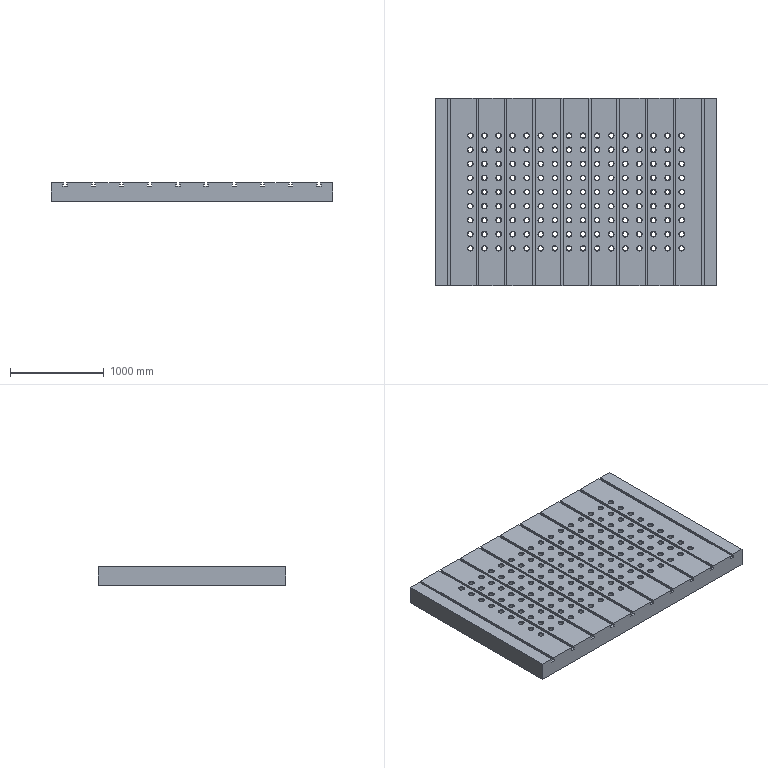Part | NX | features solid 2 | 1 solid | 518 faces | box 3000 x 2000 x 200 mm | volume 1107626279 mm3 | cylinder 288 | plane 230 | commonest cylinder face diameters 52 x144 60 x144